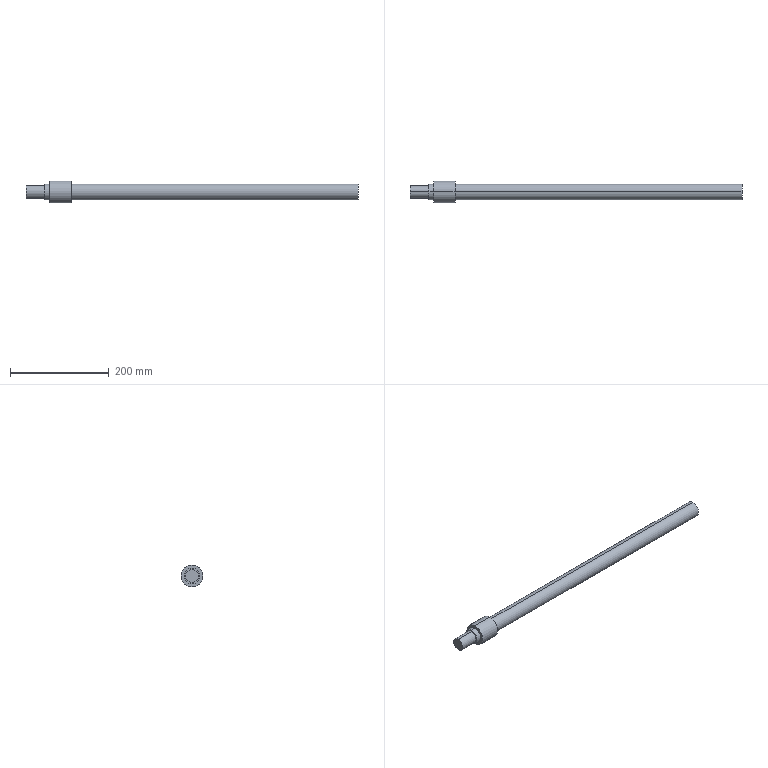Part | SolidWorks | features Revolution 1 | 1 solid | 13 faces | box 671 x 44 x 44 mm | volume 560064 mm3 | cylinder 8 | plane 5 | commonest cylinder face diameters 32 x4 26 x2 44 x2
STEP:
#1=CARTESIAN_POINT('',(562.175,0.,16.));
#2=VERTEX_POINT('',#1);
#3=CARTESIAN_POINT('',(562.175,0.,-16.));
#4=VERTEX_POINT('',#3);
#5=CARTESIAN_POINT('',(562.175,0.,0.));
#6=DIRECTION('',(-1.,0.,0.));
#7=DIRECTION('',(0.,0.,1.));
#8=AXIS2_PLACEMENT_3D('',#5,#6,#7);
#9=CIRCLE('',#8,16.);
#10=EDGE_CURVE('',#2,#4,#9,.T.);
#11=ORIENTED_EDGE('',*,*,#10,.T.);
#12=CARTESIAN_POINT('',(-17.825,0.,-16.));
#13=VERTEX_POINT('',#12);
#14=CARTESIAN_POINT('',(-119.58,0.,-16.));
#15=DIRECTION('',(-1.,0.,0.));
#16=VECTOR('',#15,1000.);
#17=LINE('',#14,#16);
#18=EDGE_CURVE('',#4,#13,#17,.T.);
#19=ORIENTED_EDGE('',*,*,#18,.T.);
#20=CARTESIAN_POINT('',(-17.825,0.,16.));
#21=VERTEX_POINT('',#20);
#22=CARTESIAN_POINT('',(-17.825,0.,0.));
#23=DIRECTION('',(-1.,0.,0.));
#24=DIRECTION('',(0.,0.,1.));
#25=AXIS2_PLACEMENT_3D('',#22,#23,#24);
#26=CIRCLE('',#25,16.);
#27=EDGE_CURVE('',#21,#13,#26,.T.);
#28=ORIENTED_EDGE('',*,*,#27,.F.);
#29=CARTESIAN_POINT('',(-119.58,0.,16.));
#30=DIRECTION('',(-1.,0.,0.));
#31=VECTOR('',#30,1000.);
#32=LINE('',#29,#31);
#33=EDGE_CURVE('',#2,#21,#32,.T.);
#34=ORIENTED_EDGE('',*,*,#33,.F.);
#35=EDGE_LOOP('',(#11,#19,#28,#34));
#36=FACE_OUTER_BOUND('',#35,.T.);
#37=CARTESIAN_POINT('',(-119.58,0.,0.));
#38=DIRECTION('',(-1.,0.,0.));
#39=DIRECTION('',(0.,0.,1.));
#40=AXIS2_PLACEMENT_3D('',#37,#38,#39);
#41=CYLINDRICAL_SURFACE('',#40,16.);
#42=ADVANCED_FACE('',(#36),#41,.T.);
#43=CARTESIAN_POINT('',(-17.825,0.,22.));
#44=VERTEX_POINT('',#43);
#45=CARTESIAN_POINT('',(-17.825,0.,-22.));
#46=VERTEX_POINT('',#45);
#47=CARTESIAN_POINT('',(-17.825,0.,0.));
#48=DIRECTION('',(-1.,0.,0.));
#49=DIRECTION('',(0.,0.,1.));
#50=AXIS2_PLACEMENT_3D('',#47,#48,#49);
#51=CIRCLE('',#50,22.);
#52=EDGE_CURVE('',#44,#46,#51,.T.);
#53=ORIENTED_EDGE('',*,*,#52,.T.);
#54=CARTESIAN_POINT('',(-60.825,0.,-22.));
#55=VERTEX_POINT('',#54);
#56=CARTESIAN_POINT('',(-119.58,0.,-22.));
#57=DIRECTION('',(-1.,0.,0.));
#58=VECTOR('',#57,1000.);
#59=LINE('',#56,#58);
#60=EDGE_CURVE('',#46,#55,#59,.T.);
#61=ORIENTED_EDGE('',*,*,#60,.T.);
#62=CARTESIAN_POINT('',(-60.825,0.,22.));
#63=VERTEX_POINT('',#62);
#64=CARTESIAN_POINT('',(-60.825,0.,0.));
#65=DIRECTION('',(-1.,0.,0.));
#66=DIRECTION('',(0.,0.,1.));
#67=AXIS2_PLACEMENT_3D('',#64,#65,#66);
#68=CIRCLE('',#67,22.);
#69=EDGE_CURVE('',#63,#55,#68,.T.);
#70=ORIENTED_EDGE('',*,*,#69,.F.);
#71=CARTESIAN_POINT('',(-119.58,0.,22.));
#72=DIRECTION('',(-1.,0.,0.));
#73=VECTOR('',#72,1000.);
#74=LINE('',#71,#73);
#75=EDGE_CURVE('',#44,#63,#74,.T.);
#76=ORIENTED_EDGE('',*,*,#75,.F.);
#77=EDGE_LOOP('',(#53,#61,#70,#76));
#78=FACE_OUTER_BOUND('',#77,.T.);
#79=CARTESIAN_POINT('',(-119.58,0.,0.));
#80=DIRECTION('',(-1.,0.,0.));
#81=DIRECTION('',(0.,0.,1.));
#82=AXIS2_PLACEMENT_3D('',#79,#80,#81);
#83=CYLINDRICAL_SURFACE('',#82,22.);
#84=ADVANCED_FACE('',(#78),#83,.T.);
#85=CARTESIAN_POINT('',(-60.825,0.,16.));
#86=VERTEX_POINT('',#85);
#87=CARTESIAN_POINT('',(-60.825,0.,-16.));
#88=VERTEX_POINT('',#87);
#89=CARTESIAN_POINT('',(-60.825,0.,0.));
#90=DIRECTION('',(-1.,0.,0.));
#91=DIRECTION('',(0.,0.,1.));
#92=AXIS2_PLACEMENT_3D('',#89,#90,#91);
#93=CIRCLE('',#92,16.);
#94=EDGE_CURVE('',#86,#88,#93,.T.);
#95=ORIENTED_EDGE('',*,*,#94,.T.);
#96=CARTESIAN_POINT('',(-70.825,0.,-16.));
#97=VERTEX_POINT('',#96);
#98=CARTESIAN_POINT('',(-119.58,0.,-16.));
#99=DIRECTION('',(-1.,0.,0.));
#100=VECTOR('',#99,1000.);
#101=LINE('',#98,#100);
#102=EDGE_CURVE('',#88,#97,#101,.T.);
#103=ORIENTED_EDGE('',*,*,#102,.T.);
#104=CARTESIAN_POINT('',(-70.825,0.,16.));
#105=VERTEX_POINT('',#104);
#106=CARTESIAN_POINT('',(-70.825,0.,0.));
#107=DIRECTION('',(-1.,0.,0.));
#108=DIRECTION('',(0.,0.,1.));
#109=AXIS2_PLACEMENT_3D('',#106,#107,#108);
#110=CIRCLE('',#109,16.);
#111=EDGE_CURVE('',#105,#97,#110,.T.);
#112=ORIENTED_EDGE('',*,*,#111,.F.);
#113=CARTESIAN_POINT('',(-119.58,0.,16.));
#114=DIRECTION('',(-1.,0.,0.));
#115=VECTOR('',#114,1000.);
#116=LINE('',#113,#115);
#117=EDGE_CURVE('',#86,#105,#116,.T.);
#118=ORIENTED_EDGE('',*,*,#117,.F.);
#119=EDGE_LOOP('',(#95,#103,#112,#118));
#120=FACE_OUTER_BOUND('',#119,.T.);
#121=CARTESIAN_POINT('',(-119.58,0.,0.));
#122=DIRECTION('',(-1.,0.,0.));
#123=DIRECTION('',(0.,0.,1.));
#124=AXIS2_PLACEMENT_3D('',#121,#122,#123);
#125=CYLINDRICAL_SURFACE('',#124,16.);
#126=ADVANCED_FACE('',(#120),#125,.T.);
#127=CARTESIAN_POINT('',(-70.825,0.,13.));
#128=VERTEX_POINT('',#127);
#129=CARTESIAN_POINT('',(-70.825,0.,-13.));
#130=VERTEX_POINT('',#129);
#131=CARTESIAN_POINT('',(-70.825,0.,0.));
#132=DIRECTION('',(-1.,0.,0.));
#133=DIRECTION('',(0.,0.,1.));
#134=AXIS2_PLACEMENT_3D('',#131,#132,#133);
#135=CIRCLE('',#134,13.);
#136=EDGE_CURVE('',#128,#130,#135,.T.);
#137=ORIENTED_EDGE('',*,*,#136,.T.);
#138=CARTESIAN_POINT('',(-108.825,0.,-13.));
#139=VERTEX_POINT('',#138);
#140=CARTESIAN_POINT('',(-119.58,0.,-13.));
#141=DIRECTION('',(-1.,0.,0.));
#142=VECTOR('',#141,1000.);
#143=LINE('',#140,#142);
#144=EDGE_CURVE('',#130,#139,#143,.T.);
#145=ORIENTED_EDGE('',*,*,#144,.T.);
#146=CARTESIAN_POINT('',(-108.825,0.,13.));
#147=VERTEX_POINT('',#146);
#148=CARTESIAN_POINT('',(-108.825,0.,0.));
#149=DIRECTION('',(-1.,0.,0.));
#150=DIRECTION('',(0.,0.,1.));
#151=AXIS2_PLACEMENT_3D('',#148,#149,#150);
#152=CIRCLE('',#151,13.);
#153=EDGE_CURVE('',#147,#139,#152,.T.);
#154=ORIENTED_EDGE('',*,*,#153,.F.);
#155=CARTESIAN_POINT('',(-119.58,0.,13.));
#156=DIRECTION('',(-1.,0.,0.));
#157=VECTOR('',#156,1000.);
#158=LINE('',#155,#157);
#159=EDGE_CURVE('',#128,#147,#158,.T.);
#160=ORIENTED_EDGE('',*,*,#159,.F.);
#161=EDGE_LOOP('',(#137,#145,#154,#160));
#162=FACE_OUTER_BOUND('',#161,.T.);
#163=CARTESIAN_POINT('',(-119.58,0.,0.));
#164=DIRECTION('',(-1.,0.,0.));
#165=DIRECTION('',(0.,0.,1.));
#166=AXIS2_PLACEMENT_3D('',#163,#164,#165);
#167=CYLINDRICAL_SURFACE('',#166,13.);
#168=ADVANCED_FACE('',(#162),#167,.T.);
#169=ORIENTED_EDGE('',*,*,#153,.T.);
#170=CARTESIAN_POINT('',(-108.825,0.,0.));
#171=DIRECTION('',(-1.,0.,0.));
#172=DIRECTION('',(0.,0.,1.));
#173=AXIS2_PLACEMENT_3D('',#170,#171,#172);
#174=CIRCLE('',#173,13.);
#175=EDGE_CURVE('',#139,#147,#174,.T.);
#176=ORIENTED_EDGE('',*,*,#175,.T.);
#177=EDGE_LOOP('',(#169,#176));
#178=FACE_OUTER_BOUND('',#177,.T.);
#179=CARTESIAN_POINT('',(-108.825,0.,0.));
#180=DIRECTION('',(1.,0.,0.));
#181=DIRECTION('',(0.,0.,-1.));
#182=AXIS2_PLACEMENT_3D('',#179,#180,#181);
#183=PLANE('',#182);
#184=ADVANCED_FACE('',(#178),#183,.F.);
#185=ORIENTED_EDGE('',*,*,#144,.F.);
#186=CARTESIAN_POINT('',(-70.825,0.,0.));
#187=DIRECTION('',(-1.,0.,0.));
#188=DIRECTION('',(0.,0.,1.));
#189=AXIS2_PLACEMENT_3D('',#186,#187,#188);
#190=CIRCLE('',#189,13.);
#191=EDGE_CURVE('',#130,#128,#190,.T.);
#192=ORIENTED_EDGE('',*,*,#191,.T.);
#193=ORIENTED_EDGE('',*,*,#159,.T.);
#194=ORIENTED_EDGE('',*,*,#175,.F.);
#195=EDGE_LOOP('',(#185,#192,#193,#194));
#196=FACE_OUTER_BOUND('',#195,.T.);
#197=CARTESIAN_POINT('',(-119.58,0.,0.));
#198=DIRECTION('',(-1.,0.,0.));
#199=DIRECTION('',(0.,0.,1.));
#200=AXIS2_PLACEMENT_3D('',#197,#198,#199);
#201=CYLINDRICAL_SURFACE('',#200,13.);
#202=ADVANCED_FACE('',(#196),#201,.T.);
#203=ORIENTED_EDGE('',*,*,#136,.F.);
#204=ORIENTED_EDGE('',*,*,#191,.F.);
#205=EDGE_LOOP('',(#203,#204));
#206=FACE_BOUND('',#205,.T.);
#207=ORIENTED_EDGE('',*,*,#111,.T.);
#208=CARTESIAN_POINT('',(-70.825,0.,0.));
#209=DIRECTION('',(-1.,0.,0.));
#210=DIRECTION('',(0.,0.,1.));
#211=AXIS2_PLACEMENT_3D('',#208,#209,#210);
#212=CIRCLE('',#211,16.);
#213=EDGE_CURVE('',#97,#105,#212,.T.);
#214=ORIENTED_EDGE('',*,*,#213,.T.);
#215=EDGE_LOOP('',(#207,#214));
#216=FACE_OUTER_BOUND('',#215,.T.);
#217=CARTESIAN_POINT('',(-70.825,13.,0.));
#218=DIRECTION('',(1.,0.,0.));
#219=DIRECTION('',(0.,0.,-1.));
#220=AXIS2_PLACEMENT_3D('',#217,#218,#219);
#221=PLANE('',#220);
#222=ADVANCED_FACE('',(#206,#216),#221,.F.);
#223=ORIENTED_EDGE('',*,*,#102,.F.);
#224=CARTESIAN_POINT('',(-60.825,0.,0.));
#225=DIRECTION('',(-1.,0.,0.));
#226=DIRECTION('',(0.,0.,1.));
#227=AXIS2_PLACEMENT_3D('',#224,#225,#226);
#228=CIRCLE('',#227,16.);
#229=EDGE_CURVE('',#88,#86,#228,.T.);
#230=ORIENTED_EDGE('',*,*,#229,.T.);
#231=ORIENTED_EDGE('',*,*,#117,.T.);
#232=ORIENTED_EDGE('',*,*,#213,.F.);
#233=EDGE_LOOP('',(#223,#230,#231,#232));
#234=FACE_OUTER_BOUND('',#233,.T.);
#235=CARTESIAN_POINT('',(-119.58,0.,0.));
#236=DIRECTION('',(-1.,0.,0.));
#237=DIRECTION('',(0.,0.,1.));
#238=AXIS2_PLACEMENT_3D('',#235,#236,#237);
#239=CYLINDRICAL_SURFACE('',#238,16.);
#240=ADVANCED_FACE('',(#234),#239,.T.);
#241=ORIENTED_EDGE('',*,*,#94,.F.);
#242=ORIENTED_EDGE('',*,*,#229,.F.);
#243=EDGE_LOOP('',(#241,#242));
#244=FACE_BOUND('',#243,.T.);
#245=ORIENTED_EDGE('',*,*,#69,.T.);
#246=CARTESIAN_POINT('',(-60.825,0.,0.));
#247=DIRECTION('',(-1.,0.,0.));
#248=DIRECTION('',(0.,0.,1.));
#249=AXIS2_PLACEMENT_3D('',#246,#247,#248);
#250=CIRCLE('',#249,22.);
#251=EDGE_CURVE('',#55,#63,#250,.T.);
#252=ORIENTED_EDGE('',*,*,#251,.T.);
#253=EDGE_LOOP('',(#245,#252));
#254=FACE_OUTER_BOUND('',#253,.T.);
#255=CARTESIAN_POINT('',(-60.825,16.,0.));
#256=DIRECTION('',(1.,0.,0.));
#257=DIRECTION('',(0.,0.,-1.));
#258=AXIS2_PLACEMENT_3D('',#255,#256,#257);
#259=PLANE('',#258);
#260=ADVANCED_FACE('',(#244,#254),#259,.F.);
#261=ORIENTED_EDGE('',*,*,#60,.F.);
#262=CARTESIAN_POINT('',(-17.825,0.,0.));
#263=DIRECTION('',(-1.,0.,0.));
#264=DIRECTION('',(0.,0.,1.));
#265=AXIS2_PLACEMENT_3D('',#262,#263,#264);
#266=CIRCLE('',#265,22.);
#267=EDGE_CURVE('',#46,#44,#266,.T.);
#268=ORIENTED_EDGE('',*,*,#267,.T.);
#269=ORIENTED_EDGE('',*,*,#75,.T.);
#270=ORIENTED_EDGE('',*,*,#251,.F.);
#271=EDGE_LOOP('',(#261,#268,#269,#270));
#272=FACE_OUTER_BOUND('',#271,.T.);
#273=CARTESIAN_POINT('',(-119.58,0.,0.));
#274=DIRECTION('',(-1.,0.,0.));
#275=DIRECTION('',(0.,0.,1.));
#276=AXIS2_PLACEMENT_3D('',#273,#274,#275);
#277=CYLINDRICAL_SURFACE('',#276,22.);
#278=ADVANCED_FACE('',(#272),#277,.T.);
#279=ORIENTED_EDGE('',*,*,#52,.F.);
#280=ORIENTED_EDGE('',*,*,#267,.F.);
#281=EDGE_LOOP('',(#279,#280));
#282=FACE_OUTER_BOUND('',#281,.T.);
#283=ORIENTED_EDGE('',*,*,#27,.T.);
#284=CARTESIAN_POINT('',(-17.825,0.,0.));
#285=DIRECTION('',(-1.,0.,0.));
#286=DIRECTION('',(0.,0.,1.));
#287=AXIS2_PLACEMENT_3D('',#284,#285,#286);
#288=CIRCLE('',#287,16.);
#289=EDGE_CURVE('',#13,#21,#288,.T.);
#290=ORIENTED_EDGE('',*,*,#289,.T.);
#291=EDGE_LOOP('',(#283,#290));
#292=FACE_BOUND('',#291,.T.);
#293=CARTESIAN_POINT('',(-17.825,22.,0.));
#294=DIRECTION('',(-1.,0.,0.));
#295=DIRECTION('',(0.,0.,1.));
#296=AXIS2_PLACEMENT_3D('',#293,#294,#295);
#297=PLANE('',#296);
#298=ADVANCED_FACE('',(#282,#292),#297,.F.);
#299=ORIENTED_EDGE('',*,*,#18,.F.);
#300=CARTESIAN_POINT('',(562.175,0.,0.));
#301=DIRECTION('',(-1.,0.,0.));
#302=DIRECTION('',(0.,0.,1.));
#303=AXIS2_PLACEMENT_3D('',#300,#301,#302);
#304=CIRCLE('',#303,16.);
#305=EDGE_CURVE('',#4,#2,#304,.T.);
#306=ORIENTED_EDGE('',*,*,#305,.T.);
#307=ORIENTED_EDGE('',*,*,#33,.T.);
#308=ORIENTED_EDGE('',*,*,#289,.F.);
#309=EDGE_LOOP('',(#299,#306,#307,#308));
#310=FACE_OUTER_BOUND('',#309,.T.);
#311=CARTESIAN_POINT('',(-119.58,0.,0.));
#312=DIRECTION('',(-1.,0.,0.));
#313=DIRECTION('',(0.,0.,1.));
#314=AXIS2_PLACEMENT_3D('',#311,#312,#313);
#315=CYLINDRICAL_SURFACE('',#314,16.);
#316=ADVANCED_FACE('',(#310),#315,.T.);
#317=ORIENTED_EDGE('',*,*,#10,.F.);
#318=ORIENTED_EDGE('',*,*,#305,.F.);
#319=EDGE_LOOP('',(#317,#318));
#320=FACE_OUTER_BOUND('',#319,.T.);
#321=CARTESIAN_POINT('',(562.175,16.,0.));
#322=DIRECTION('',(-1.,0.,0.));
#323=DIRECTION('',(0.,0.,1.));
#324=AXIS2_PLACEMENT_3D('',#321,#322,#323);
#325=PLANE('',#324);
#326=ADVANCED_FACE('',(#320),#325,.F.);
#327=CLOSED_SHELL('',(#42,#84,#126,#168,#184,#202,#222,#240,#260,#278,#298,#316,#326));
#328=MANIFOLD_SOLID_BREP('',#327);
#329=CARTESIAN_POINT('',(0.,0.,0.));
#330=DIRECTION('',(0.,0.,1.));
#331=DIRECTION('',(1.,0.,0.));
#332=AXIS2_PLACEMENT_3D('',#329,#330,#331);
#333=(LENGTH_UNIT()NAMED_UNIT(*)SI_UNIT(.MILLI.,.METRE.));
#334=UNCERTAINTY_MEASURE_WITH_UNIT(LENGTH_MEASURE(0.00001),#333,'','');
#335=(NAMED_UNIT(*)PLANE_ANGLE_UNIT()SI_UNIT($,.RADIAN.));
#336=(NAMED_UNIT(*)SI_UNIT($,.STERADIAN.)SOLID_ANGLE_UNIT());
#337=(GEOMETRIC_REPRESENTATION_CONTEXT(3)GLOBAL_UNCERTAINTY_ASSIGNED_CONTEXT((#334))GLOBAL_UNIT_ASSIGNED_CONTEXT((#333,#335,#336))REPRESENTATION_CONTEXT('',''));
#338=ADVANCED_BREP_SHAPE_REPRESENTATION('',(#328,#332),#337);